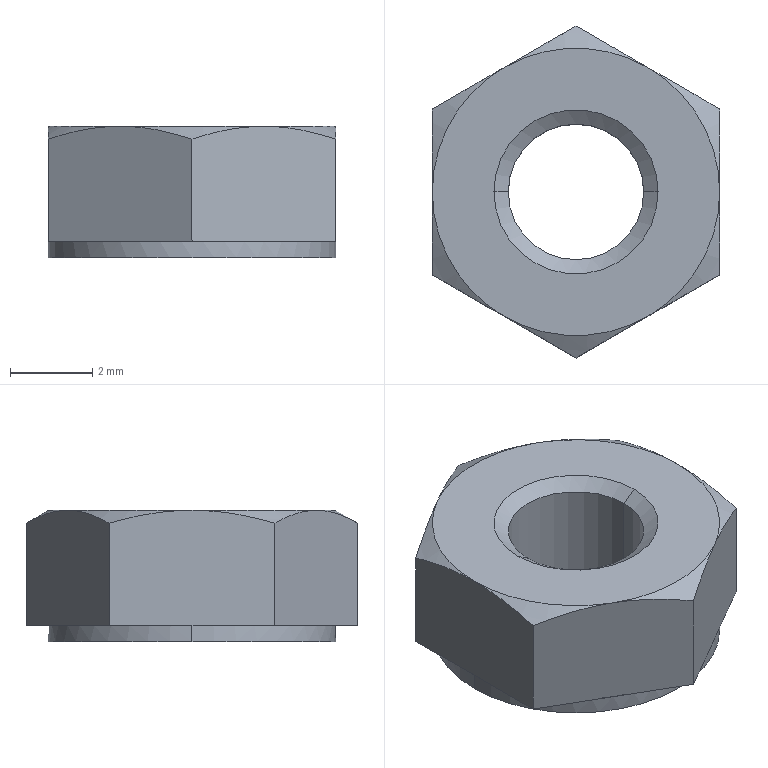Part | SolidWorks | features RevCut 4, Extrusion 1, LPattern 1 | 1 solid | 30 faces | box 7 x 8.083 x 3.2 mm | volume 105.415 mm3 | plane 14 | cone 10 | cylinder 6 | commonest cylinder face diameters 3.3 x2 4 x2 7 x2
STEP:
#1=CARTESIAN_POINT('',(-2.,0.,-3.2));
#2=VERTEX_POINT('',#1);
#3=CARTESIAN_POINT('',(2.,0.,-3.2));
#4=VERTEX_POINT('',#3);
#5=CARTESIAN_POINT('',(0.,0.,-3.2));
#6=DIRECTION('',(0.,0.,1.));
#7=DIRECTION('',(-1.,0.,0.));
#8=AXIS2_PLACEMENT_3D('',#5,#6,#7);
#9=CIRCLE('',#8,2.);
#10=EDGE_CURVE('',#2,#4,#9,.T.);
#11=ORIENTED_EDGE('',*,*,#10,.F.);
#12=CARTESIAN_POINT('',(-2.,0.,-3.175));
#13=VERTEX_POINT('',#12);
#14=CARTESIAN_POINT('',(-2.,0.,-25.038));
#15=DIRECTION('',(0.,0.,1.));
#16=VECTOR('',#15,1000.);
#17=LINE('',#14,#16);
#18=EDGE_CURVE('',#2,#13,#17,.T.);
#19=ORIENTED_EDGE('',*,*,#18,.T.);
#20=CARTESIAN_POINT('',(2.,0.,-3.175));
#21=VERTEX_POINT('',#20);
#22=CARTESIAN_POINT('',(0.,0.,-3.175));
#23=DIRECTION('',(0.,0.,1.));
#24=DIRECTION('',(1.,0.,0.));
#25=AXIS2_PLACEMENT_3D('',#22,#23,#24);
#26=CIRCLE('',#25,2.);
#27=EDGE_CURVE('',#13,#21,#26,.T.);
#28=ORIENTED_EDGE('',*,*,#27,.T.);
#29=CARTESIAN_POINT('',(2.,0.,-25.038));
#30=DIRECTION('',(0.,0.,1.));
#31=VECTOR('',#30,1000.);
#32=LINE('',#29,#31);
#33=EDGE_CURVE('',#4,#21,#32,.T.);
#34=ORIENTED_EDGE('',*,*,#33,.F.);
#35=EDGE_LOOP('',(#11,#19,#28,#34));
#36=FACE_OUTER_BOUND('',#35,.T.);
#37=CARTESIAN_POINT('',(0.,0.,-25.038));
#38=DIRECTION('',(0.,0.,1.));
#39=DIRECTION('',(1.,0.,0.));
#40=AXIS2_PLACEMENT_3D('',#37,#38,#39);
#41=CYLINDRICAL_SURFACE('',#40,2.);
#42=ADVANCED_FACE('',(#36),#41,.F.);
#43=CARTESIAN_POINT('',(-1.65,0.,-2.93));
#44=VERTEX_POINT('',#43);
#45=CARTESIAN_POINT('',(1.65,0.,-2.93));
#46=VERTEX_POINT('',#45);
#47=CARTESIAN_POINT('',(0.,0.,-2.93));
#48=DIRECTION('',(0.,0.,1.));
#49=DIRECTION('',(-1.,0.,0.));
#50=AXIS2_PLACEMENT_3D('',#47,#48,#49);
#51=CIRCLE('',#50,1.65);
#52=EDGE_CURVE('',#44,#46,#51,.T.);
#53=ORIENTED_EDGE('',*,*,#52,.T.);
#54=CARTESIAN_POINT('',(2.,0.,-3.175));
#55=DIRECTION('',(0.8192,0.,-0.5736));
#56=VECTOR('',#55,1000.);
#57=LINE('',#54,#56);
#58=EDGE_CURVE('',#46,#21,#57,.T.);
#59=ORIENTED_EDGE('',*,*,#58,.T.);
#60=ORIENTED_EDGE('',*,*,#27,.F.);
#61=CARTESIAN_POINT('',(-2.,0.,-3.175));
#62=DIRECTION('',(-0.8192,0.,-0.5736));
#63=VECTOR('',#62,1000.);
#64=LINE('',#61,#63);
#65=EDGE_CURVE('',#44,#13,#64,.T.);
#66=ORIENTED_EDGE('',*,*,#65,.F.);
#67=EDGE_LOOP('',(#53,#59,#60,#66));
#68=FACE_OUTER_BOUND('',#67,.T.);
#69=CARTESIAN_POINT('',(0.,0.,-3.175));
#70=DIRECTION('',(0.,0.,-1.));
#71=DIRECTION('',(-1.,0.,0.));
#72=AXIS2_PLACEMENT_3D('',#69,#70,#71);
#73=CONICAL_SURFACE('',#72,2.,0.9599);
#74=ADVANCED_FACE('',(#68),#73,.F.);
#75=CARTESIAN_POINT('',(1.65,0.,-0.2451));
#76=VERTEX_POINT('',#75);
#77=CARTESIAN_POINT('',(-1.65,0.,-0.2451));
#78=VERTEX_POINT('',#77);
#79=CARTESIAN_POINT('',(0.,0.,-0.2451));
#80=DIRECTION('',(0.,0.,-1.));
#81=DIRECTION('',(1.,0.,0.));
#82=AXIS2_PLACEMENT_3D('',#79,#80,#81);
#83=CIRCLE('',#82,1.65);
#84=EDGE_CURVE('',#76,#78,#83,.T.);
#85=ORIENTED_EDGE('',*,*,#84,.T.);
#86=CARTESIAN_POINT('',(-2.,0.,0.));
#87=VERTEX_POINT('',#86);
#88=CARTESIAN_POINT('',(-1.615,0.,-0.2696));
#89=DIRECTION('',(-0.8192,0.,0.5736));
#90=VECTOR('',#89,1000.);
#91=LINE('',#88,#90);
#92=EDGE_CURVE('',#78,#87,#91,.T.);
#93=ORIENTED_EDGE('',*,*,#92,.T.);
#94=CARTESIAN_POINT('',(2.,0.,0.));
#95=VERTEX_POINT('',#94);
#96=CARTESIAN_POINT('',(0.,0.,0.));
#97=DIRECTION('',(0.,0.,1.));
#98=DIRECTION('',(1.,0.,0.));
#99=AXIS2_PLACEMENT_3D('',#96,#97,#98);
#100=CIRCLE('',#99,2.);
#101=EDGE_CURVE('',#87,#95,#100,.T.);
#102=ORIENTED_EDGE('',*,*,#101,.T.);
#103=CARTESIAN_POINT('',(1.615,0.,-0.2696));
#104=DIRECTION('',(0.8192,0.,0.5736));
#105=VECTOR('',#104,1000.);
#106=LINE('',#103,#105);
#107=EDGE_CURVE('',#76,#95,#106,.T.);
#108=ORIENTED_EDGE('',*,*,#107,.F.);
#109=EDGE_LOOP('',(#85,#93,#102,#108));
#110=FACE_OUTER_BOUND('',#109,.T.);
#111=CARTESIAN_POINT('',(0.,0.,-0.2696));
#112=DIRECTION('',(0.,0.,1.));
#113=DIRECTION('',(1.,0.,0.));
#114=AXIS2_PLACEMENT_3D('',#111,#112,#113);
#115=CONICAL_SURFACE('',#114,1.615,0.9599);
#116=ADVANCED_FACE('',(#110),#115,.F.);
#117=CARTESIAN_POINT('',(3.5,0.,-3.2));
#118=VERTEX_POINT('',#117);
#119=CARTESIAN_POINT('',(-3.5,0.,-3.2));
#120=VERTEX_POINT('',#119);
#121=CARTESIAN_POINT('',(0.,0.,-3.2));
#122=DIRECTION('',(0.,0.,1.));
#123=DIRECTION('',(-1.,0.,0.));
#124=AXIS2_PLACEMENT_3D('',#121,#122,#123);
#125=CIRCLE('',#124,3.5);
#126=EDGE_CURVE('',#118,#120,#125,.T.);
#127=ORIENTED_EDGE('',*,*,#126,.T.);
#128=CARTESIAN_POINT('',(-3.5,0.,-2.8));
#129=VERTEX_POINT('',#128);
#130=CARTESIAN_POINT('',(-3.5,0.,0.));
#131=DIRECTION('',(0.,0.,1.));
#132=VECTOR('',#131,1000.);
#133=LINE('',#130,#132);
#134=EDGE_CURVE('',#120,#129,#133,.T.);
#135=ORIENTED_EDGE('',*,*,#134,.T.);
#136=CARTESIAN_POINT('',(-1.75,3.031,-2.8));
#137=VERTEX_POINT('',#136);
#138=CARTESIAN_POINT('',(0.,0.,-2.8));
#139=DIRECTION('',(0.,0.,1.));
#140=DIRECTION('',(1.,0.,0.));
#141=AXIS2_PLACEMENT_3D('',#138,#139,#140);
#142=CIRCLE('',#141,3.5);
#143=EDGE_CURVE('',#137,#129,#142,.T.);
#144=ORIENTED_EDGE('',*,*,#143,.F.);
#145=CARTESIAN_POINT('',(1.75,3.031,-2.8));
#146=VERTEX_POINT('',#145);
#147=CARTESIAN_POINT('',(0.,0.,-2.8));
#148=DIRECTION('',(0.,0.,1.));
#149=DIRECTION('',(1.,0.,0.));
#150=AXIS2_PLACEMENT_3D('',#147,#148,#149);
#151=CIRCLE('',#150,3.5);
#152=EDGE_CURVE('',#146,#137,#151,.T.);
#153=ORIENTED_EDGE('',*,*,#152,.F.);
#154=CARTESIAN_POINT('',(3.5,0.,-2.8));
#155=VERTEX_POINT('',#154);
#156=CARTESIAN_POINT('',(0.,0.,-2.8));
#157=DIRECTION('',(0.,0.,1.));
#158=DIRECTION('',(1.,0.,0.));
#159=AXIS2_PLACEMENT_3D('',#156,#157,#158);
#160=CIRCLE('',#159,3.5);
#161=EDGE_CURVE('',#155,#146,#160,.T.);
#162=ORIENTED_EDGE('',*,*,#161,.F.);
#163=CARTESIAN_POINT('',(3.5,0.,0.));
#164=DIRECTION('',(0.,0.,1.));
#165=VECTOR('',#164,1000.);
#166=LINE('',#163,#165);
#167=EDGE_CURVE('',#118,#155,#166,.T.);
#168=ORIENTED_EDGE('',*,*,#167,.F.);
#169=EDGE_LOOP('',(#127,#135,#144,#153,#162,#168));
#170=FACE_OUTER_BOUND('',#169,.T.);
#171=CARTESIAN_POINT('',(0.,0.,0.));
#172=DIRECTION('',(0.,0.,1.));
#173=DIRECTION('',(1.,0.,0.));
#174=AXIS2_PLACEMENT_3D('',#171,#172,#173);
#175=CYLINDRICAL_SURFACE('',#174,3.5);
#176=ADVANCED_FACE('',(#170),#175,.T.);
#177=ORIENTED_EDGE('',*,*,#52,.F.);
#178=CARTESIAN_POINT('',(-1.65,0.,-3.2));
#179=DIRECTION('',(0.,0.,1.));
#180=VECTOR('',#179,1000.);
#181=LINE('',#178,#180);
#182=EDGE_CURVE('',#44,#78,#181,.T.);
#183=ORIENTED_EDGE('',*,*,#182,.T.);
#184=ORIENTED_EDGE('',*,*,#84,.F.);
#185=CARTESIAN_POINT('',(1.65,0.,-3.2));
#186=DIRECTION('',(0.,0.,1.));
#187=VECTOR('',#186,1000.);
#188=LINE('',#185,#187);
#189=EDGE_CURVE('',#46,#76,#188,.T.);
#190=ORIENTED_EDGE('',*,*,#189,.F.);
#191=EDGE_LOOP('',(#177,#183,#184,#190));
#192=FACE_OUTER_BOUND('',#191,.T.);
#193=CARTESIAN_POINT('',(0.,0.,-3.2));
#194=DIRECTION('',(0.,0.,1.));
#195=DIRECTION('',(1.,0.,0.));
#196=AXIS2_PLACEMENT_3D('',#193,#194,#195);
#197=CYLINDRICAL_SURFACE('',#196,1.65);
#198=ADVANCED_FACE('',(#192),#197,.F.);
#199=ORIENTED_EDGE('',*,*,#182,.F.);
#200=CARTESIAN_POINT('',(0.,0.,-2.93));
#201=DIRECTION('',(0.,0.,1.));
#202=DIRECTION('',(-1.,0.,0.));
#203=AXIS2_PLACEMENT_3D('',#200,#201,#202);
#204=CIRCLE('',#203,1.65);
#205=EDGE_CURVE('',#46,#44,#204,.T.);
#206=ORIENTED_EDGE('',*,*,#205,.F.);
#207=ORIENTED_EDGE('',*,*,#189,.T.);
#208=CARTESIAN_POINT('',(0.,0.,-0.2451));
#209=DIRECTION('',(0.,0.,-1.));
#210=DIRECTION('',(1.,0.,0.));
#211=AXIS2_PLACEMENT_3D('',#208,#209,#210);
#212=CIRCLE('',#211,1.65);
#213=EDGE_CURVE('',#78,#76,#212,.T.);
#214=ORIENTED_EDGE('',*,*,#213,.F.);
#215=EDGE_LOOP('',(#199,#206,#207,#214));
#216=FACE_OUTER_BOUND('',#215,.T.);
#217=CARTESIAN_POINT('',(0.,0.,-3.2));
#218=DIRECTION('',(0.,0.,1.));
#219=DIRECTION('',(1.,0.,0.));
#220=AXIS2_PLACEMENT_3D('',#217,#218,#219);
#221=CYLINDRICAL_SURFACE('',#220,1.65);
#222=ADVANCED_FACE('',(#216),#221,.F.);
#223=CARTESIAN_POINT('',(-3.5,2.021,-2.8));
#224=VERTEX_POINT('',#223);
#225=CARTESIAN_POINT('',(-3.5,2.021,-0.3126));
#226=VERTEX_POINT('',#225);
#227=CARTESIAN_POINT('',(-3.5,2.021,-3.2));
#228=DIRECTION('',(0.,0.,1.));
#229=VECTOR('',#228,1000.);
#230=LINE('',#227,#229);
#231=EDGE_CURVE('',#224,#226,#230,.T.);
#232=ORIENTED_EDGE('',*,*,#231,.T.);
#233=CARTESIAN_POINT('',(-1.75,3.031,0.));
#234=VERTEX_POINT('',#233);
#235=CARTESIAN_POINT('',(-3.5,2.021,-0.3126));
#236=CARTESIAN_POINT('',(-2.927,2.351,-0.1218));
#237=CARTESIAN_POINT('',(-2.346,2.687,0.));
#238=CARTESIAN_POINT('',(-1.75,3.031,0.));
#239=B_SPLINE_CURVE_WITH_KNOTS('',3,(#235,#236,#237,#238),.UNSPECIFIED.,.F.,.F.,(4,4),(0.000000238,0.002045),.UNSPECIFIED.);
#240=EDGE_CURVE('',#226,#234,#239,.T.);
#241=ORIENTED_EDGE('',*,*,#240,.T.);
#242=CARTESIAN_POINT('',(0.,4.041,-0.3126));
#243=VERTEX_POINT('',#242);
#244=CARTESIAN_POINT('',(-1.75,3.031,0.));
#245=CARTESIAN_POINT('',(-1.453,3.203,0.));
#246=CARTESIAN_POINT('',(-1.156,3.374,-0.02993));
#247=CARTESIAN_POINT('',(-0.5735,3.71,-0.1388));
#248=CARTESIAN_POINT('',(-0.2856,3.877,-0.2174));
#249=CARTESIAN_POINT('',(0.,4.041,-0.3126));
#250=B_SPLINE_CURVE_WITH_KNOTS('',3,(#244,#245,#246,#247,#248,#249),.UNSPECIFIED.,.F.,.F.,(4,2,4),(0.002045,0.003063,0.004082),.UNSPECIFIED.);
#251=EDGE_CURVE('',#234,#243,#250,.T.);
#252=ORIENTED_EDGE('',*,*,#251,.T.);
#253=CARTESIAN_POINT('',(0.,4.041,-2.8));
#254=VERTEX_POINT('',#253);
#255=CARTESIAN_POINT('',(0.,4.041,-3.2));
#256=DIRECTION('',(0.,0.,1.));
#257=VECTOR('',#256,1000.);
#258=LINE('',#255,#257);
#259=EDGE_CURVE('',#254,#243,#258,.T.);
#260=ORIENTED_EDGE('',*,*,#259,.F.);
#261=CARTESIAN_POINT('',(0.,4.041,-2.8));
#262=DIRECTION('',(-0.866,-0.5,0.));
#263=VECTOR('',#262,1000.);
#264=LINE('',#261,#263);
#265=EDGE_CURVE('',#254,#137,#264,.T.);
#266=ORIENTED_EDGE('',*,*,#265,.T.);
#267=CARTESIAN_POINT('',(0.,4.041,-2.8));
#268=DIRECTION('',(-0.866,-0.5,0.));
#269=VECTOR('',#268,1000.);
#270=LINE('',#267,#269);
#271=EDGE_CURVE('',#137,#224,#270,.T.);
#272=ORIENTED_EDGE('',*,*,#271,.T.);
#273=EDGE_LOOP('',(#232,#241,#252,#260,#266,#272));
#274=FACE_OUTER_BOUND('',#273,.T.);
#275=CARTESIAN_POINT('',(0.,4.041,-3.2));
#276=DIRECTION('',(-0.5,0.866,0.));
#277=DIRECTION('',(-0.866,-0.5,0.));
#278=AXIS2_PLACEMENT_3D('',#275,#276,#277);
#279=PLANE('',#278);
#280=ADVANCED_FACE('',(#274),#279,.T.);
#281=ORIENTED_EDGE('',*,*,#259,.T.);
#282=CARTESIAN_POINT('',(1.75,3.031,0.));
#283=VERTEX_POINT('',#282);
#284=CARTESIAN_POINT('',(0.,4.041,-0.3126));
#285=CARTESIAN_POINT('',(0.5726,3.711,-0.1218));
#286=CARTESIAN_POINT('',(1.154,3.375,0.));
#287=CARTESIAN_POINT('',(1.75,3.031,0.));
#288=B_SPLINE_CURVE_WITH_KNOTS('',3,(#284,#285,#286,#287),.UNSPECIFIED.,.F.,.F.,(4,4),(0.000000238,0.002045),.UNSPECIFIED.);
#289=EDGE_CURVE('',#243,#283,#288,.T.);
#290=ORIENTED_EDGE('',*,*,#289,.T.);
#291=CARTESIAN_POINT('',(3.5,2.021,-0.3126));
#292=VERTEX_POINT('',#291);
#293=CARTESIAN_POINT('',(1.75,3.031,0.));
#294=CARTESIAN_POINT('',(2.047,2.86,0.));
#295=CARTESIAN_POINT('',(2.344,2.688,-0.02993));
#296=CARTESIAN_POINT('',(2.926,2.352,-0.1388));
#297=CARTESIAN_POINT('',(3.214,2.186,-0.2174));
#298=CARTESIAN_POINT('',(3.5,2.021,-0.3126));
#299=B_SPLINE_CURVE_WITH_KNOTS('',3,(#293,#294,#295,#296,#297,#298),.UNSPECIFIED.,.F.,.F.,(4,2,4),(0.002045,0.003063,0.004082),.UNSPECIFIED.);
#300=EDGE_CURVE('',#283,#292,#299,.T.);
#301=ORIENTED_EDGE('',*,*,#300,.T.);
#302=CARTESIAN_POINT('',(3.5,2.021,-2.8));
#303=VERTEX_POINT('',#302);
#304=CARTESIAN_POINT('',(3.5,2.021,-3.2));
#305=DIRECTION('',(0.,0.,1.));
#306=VECTOR('',#305,1000.);
#307=LINE('',#304,#306);
#308=EDGE_CURVE('',#303,#292,#307,.T.);
#309=ORIENTED_EDGE('',*,*,#308,.F.);
#310=CARTESIAN_POINT('',(3.5,2.021,-2.8));
#311=DIRECTION('',(-0.866,0.5,0.));
#312=VECTOR('',#311,1000.);
#313=LINE('',#310,#312);
#314=EDGE_CURVE('',#303,#146,#313,.T.);
#315=ORIENTED_EDGE('',*,*,#314,.T.);
#316=CARTESIAN_POINT('',(3.5,2.021,-2.8));
#317=DIRECTION('',(-0.866,0.5,0.));
#318=VECTOR('',#317,1000.);
#319=LINE('',#316,#318);
#320=EDGE_CURVE('',#146,#254,#319,.T.);
#321=ORIENTED_EDGE('',*,*,#320,.T.);
#322=EDGE_LOOP('',(#281,#290,#301,#309,#315,#321));
#323=FACE_OUTER_BOUND('',#322,.T.);
#324=CARTESIAN_POINT('',(3.5,2.021,-3.2));
#325=DIRECTION('',(0.5,0.866,0.));
#326=DIRECTION('',(-0.866,0.5,0.));
#327=AXIS2_PLACEMENT_3D('',#324,#325,#326);
#328=PLANE('',#327);
#329=ADVANCED_FACE('',(#323),#328,.T.);
#330=CARTESIAN_POINT('',(3.5,-2.021,-0.3126));
#331=VERTEX_POINT('',#330);
#332=CARTESIAN_POINT('',(3.5,0.,0.));
#333=VERTEX_POINT('',#332);
#334=CARTESIAN_POINT('',(3.5,-2.021,-0.3126));
#335=CARTESIAN_POINT('',(3.5,-1.692,-0.2177));
#336=CARTESIAN_POINT('',(3.5,-1.355,-0.1382));
#337=CARTESIAN_POINT('',(3.5,-0.6807,-0.02935));
#338=CARTESIAN_POINT('',(3.5,-0.3415,0.));
#339=CARTESIAN_POINT('',(3.5,0.,0.));
#340=B_SPLINE_CURVE_WITH_KNOTS('',3,(#334,#335,#336,#337,#338,#339),.UNSPECIFIED.,.F.,.F.,(4,2,4),(0.003605,0.004627,0.005649),.UNSPECIFIED.);
#341=EDGE_CURVE('',#331,#333,#340,.T.);
#342=ORIENTED_EDGE('',*,*,#341,.F.);
#343=CARTESIAN_POINT('',(3.5,-2.021,-2.8));
#344=VERTEX_POINT('',#343);
#345=CARTESIAN_POINT('',(3.5,-2.021,-3.2));
#346=DIRECTION('',(0.,0.,1.));
#347=VECTOR('',#346,1000.);
#348=LINE('',#345,#347);
#349=EDGE_CURVE('',#344,#331,#348,.T.);
#350=ORIENTED_EDGE('',*,*,#349,.F.);
#351=CARTESIAN_POINT('',(3.5,2.021,-2.8));
#352=DIRECTION('',(0.,-1.,0.));
#353=VECTOR('',#352,1000.);
#354=LINE('',#351,#353);
#355=EDGE_CURVE('',#155,#344,#354,.T.);
#356=ORIENTED_EDGE('',*,*,#355,.F.);
#357=CARTESIAN_POINT('',(3.5,2.021,-2.8));
#358=DIRECTION('',(0.,-1.,0.));
#359=VECTOR('',#358,1000.);
#360=LINE('',#357,#359);
#361=EDGE_CURVE('',#303,#155,#360,.T.);
#362=ORIENTED_EDGE('',*,*,#361,.F.);
#363=ORIENTED_EDGE('',*,*,#308,.T.);
#364=CARTESIAN_POINT('',(3.5,0.,0.));
#365=CARTESIAN_POINT('',(3.5,0.3417,0.));
#366=CARTESIAN_POINT('',(3.5,0.688,-0.03016));
#367=CARTESIAN_POINT('',(3.5,1.363,-0.1397));
#368=CARTESIAN_POINT('',(3.5,1.694,-0.2183));
#369=CARTESIAN_POINT('',(3.5,2.021,-0.3126));
#370=B_SPLINE_CURVE_WITH_KNOTS('',3,(#364,#365,#366,#367,#368,#369),.UNSPECIFIED.,.F.,.F.,(4,2,4),(0.005649,0.006672,0.007695),.UNSPECIFIED.);
#371=EDGE_CURVE('',#333,#292,#370,.T.);
#372=ORIENTED_EDGE('',*,*,#371,.F.);
#373=EDGE_LOOP('',(#342,#350,#356,#362,#363,#372));
#374=FACE_OUTER_BOUND('',#373,.T.);
#375=CARTESIAN_POINT('',(3.5,2.021,-3.2));
#376=DIRECTION('',(-1.,0.,0.));
#377=DIRECTION('',(0.,0.,1.));
#378=AXIS2_PLACEMENT_3D('',#375,#376,#377);
#379=PLANE('',#378);
#380=ADVANCED_FACE('',(#374),#379,.F.);
#381=ORIENTED_EDGE('',*,*,#349,.T.);
#382=CARTESIAN_POINT('',(1.75,-3.031,0.));
#383=VERTEX_POINT('',#382);
#384=CARTESIAN_POINT('',(3.5,-2.021,-0.3126));
#385=CARTESIAN_POINT('',(2.927,-2.351,-0.1218));
#386=CARTESIAN_POINT('',(2.346,-2.687,0.));
#387=CARTESIAN_POINT('',(1.75,-3.031,0.));
#388=B_SPLINE_CURVE_WITH_KNOTS('',3,(#384,#385,#386,#387),.UNSPECIFIED.,.F.,.F.,(4,4),(0.000000238,0.002045),.UNSPECIFIED.);
#389=EDGE_CURVE('',#331,#383,#388,.T.);
#390=ORIENTED_EDGE('',*,*,#389,.T.);
#391=CARTESIAN_POINT('',(0.,-4.041,-0.3126));
#392=VERTEX_POINT('',#391);
#393=CARTESIAN_POINT('',(1.75,-3.031,0.));
#394=CARTESIAN_POINT('',(1.453,-3.203,0.));
#395=CARTESIAN_POINT('',(1.156,-3.374,-0.02993));
#396=CARTESIAN_POINT('',(0.5735,-3.71,-0.1388));
#397=CARTESIAN_POINT('',(0.2856,-3.877,-0.2174));
#398=CARTESIAN_POINT('',(0.,-4.041,-0.3126));
#399=B_SPLINE_CURVE_WITH_KNOTS('',3,(#393,#394,#395,#396,#397,#398),.UNSPECIFIED.,.F.,.F.,(4,2,4),(0.002045,0.003063,0.004082),.UNSPECIFIED.);
#400=EDGE_CURVE('',#383,#392,#399,.T.);
#401=ORIENTED_EDGE('',*,*,#400,.T.);
#402=CARTESIAN_POINT('',(0.,-4.041,-2.8));
#403=VERTEX_POINT('',#402);
#404=CARTESIAN_POINT('',(0.,-4.041,-3.2));
#405=DIRECTION('',(0.,0.,1.));
#406=VECTOR('',#405,1000.);
#407=LINE('',#404,#406);
#408=EDGE_CURVE('',#403,#392,#407,.T.);
#409=ORIENTED_EDGE('',*,*,#408,.F.);
#410=CARTESIAN_POINT('',(1.75,-3.031,-2.8));
#411=VERTEX_POINT('',#410);
#412=CARTESIAN_POINT('',(0.,-4.041,-2.8));
#413=DIRECTION('',(0.866,0.5,0.));
#414=VECTOR('',#413,1000.);
#415=LINE('',#412,#414);
#416=EDGE_CURVE('',#403,#411,#415,.T.);
#417=ORIENTED_EDGE('',*,*,#416,.T.);
#418=CARTESIAN_POINT('',(0.,-4.041,-2.8));
#419=DIRECTION('',(0.866,0.5,0.));
#420=VECTOR('',#419,1000.);
#421=LINE('',#418,#420);
#422=EDGE_CURVE('',#411,#344,#421,.T.);
#423=ORIENTED_EDGE('',*,*,#422,.T.);
#424=EDGE_LOOP('',(#381,#390,#401,#409,#417,#423));
#425=FACE_OUTER_BOUND('',#424,.T.);
#426=CARTESIAN_POINT('',(0.,-4.041,-3.2));
#427=DIRECTION('',(0.5,-0.866,0.));
#428=DIRECTION('',(0.866,0.5,0.));
#429=AXIS2_PLACEMENT_3D('',#426,#427,#428);
#430=PLANE('',#429);
#431=ADVANCED_FACE('',(#425),#430,.T.);
#432=ORIENTED_EDGE('',*,*,#408,.T.);
#433=CARTESIAN_POINT('',(-1.75,-3.031,0.));
#434=VERTEX_POINT('',#433);
#435=CARTESIAN_POINT('',(0.,-4.041,-0.3126));
#436=CARTESIAN_POINT('',(-0.5726,-3.711,-0.1218));
#437=CARTESIAN_POINT('',(-1.154,-3.375,0.));
#438=CARTESIAN_POINT('',(-1.75,-3.031,0.));
#439=B_SPLINE_CURVE_WITH_KNOTS('',3,(#435,#436,#437,#438),.UNSPECIFIED.,.F.,.F.,(4,4),(0.000000238,0.002045),.UNSPECIFIED.);
#440=EDGE_CURVE('',#392,#434,#439,.T.);
#441=ORIENTED_EDGE('',*,*,#440,.T.);
#442=CARTESIAN_POINT('',(-3.5,-2.021,-0.3126));
#443=VERTEX_POINT('',#442);
#444=CARTESIAN_POINT('',(-1.75,-3.031,0.));
#445=CARTESIAN_POINT('',(-2.047,-2.86,0.));
#446=CARTESIAN_POINT('',(-2.344,-2.688,-0.02993));
#447=CARTESIAN_POINT('',(-2.926,-2.352,-0.1388));
#448=CARTESIAN_POINT('',(-3.214,-2.186,-0.2174));
#449=CARTESIAN_POINT('',(-3.5,-2.021,-0.3126));
#450=B_SPLINE_CURVE_WITH_KNOTS('',3,(#444,#445,#446,#447,#448,#449),.UNSPECIFIED.,.F.,.F.,(4,2,4),(0.002045,0.003063,0.004082),.UNSPECIFIED.);
#451=EDGE_CURVE('',#434,#443,#450,.T.);
#452=ORIENTED_EDGE('',*,*,#451,.T.);
#453=CARTESIAN_POINT('',(-3.5,-2.021,-2.8));
#454=VERTEX_POINT('',#453);
#455=CARTESIAN_POINT('',(-3.5,-2.021,-3.2));
#456=DIRECTION('',(0.,0.,1.));
#457=VECTOR('',#456,1000.);
#458=LINE('',#455,#457);
#459=EDGE_CURVE('',#454,#443,#458,.T.);
#460=ORIENTED_EDGE('',*,*,#459,.F.);
#461=CARTESIAN_POINT('',(-1.75,-3.031,-2.8));
#462=VERTEX_POINT('',#461);
#463=CARTESIAN_POINT('',(-3.5,-2.021,-2.8));
#464=DIRECTION('',(0.866,-0.5,0.));
#465=VECTOR('',#464,1000.);
#466=LINE('',#463,#465);
#467=EDGE_CURVE('',#454,#462,#466,.T.);
#468=ORIENTED_EDGE('',*,*,#467,.T.);
#469=CARTESIAN_POINT('',(-3.5,-2.021,-2.8));
#470=DIRECTION('',(0.866,-0.5,0.));
#471=VECTOR('',#470,1000.);
#472=LINE('',#469,#471);
#473=EDGE_CURVE('',#462,#403,#472,.T.);
#474=ORIENTED_EDGE('',*,*,#473,.T.);
#475=EDGE_LOOP('',(#432,#441,#452,#460,#468,#474));
#476=FACE_OUTER_BOUND('',#475,.T.);
#477=CARTESIAN_POINT('',(-3.5,-2.021,-3.2));
#478=DIRECTION('',(-0.5,-0.866,0.));
#479=DIRECTION('',(0.866,-0.5,0.));
#480=AXIS2_PLACEMENT_3D('',#477,#478,#479);
#481=PLANE('',#480);
#482=ADVANCED_FACE('',(#476),#481,.T.);
#483=ORIENTED_EDGE('',*,*,#459,.T.);
#484=CARTESIAN_POINT('',(-3.5,0.,0.));
#485=VERTEX_POINT('',#484);
#486=CARTESIAN_POINT('',(-3.5,-2.021,-0.3126));
#487=CARTESIAN_POINT('',(-3.5,-1.692,-0.2177));
#488=CARTESIAN_POINT('',(-3.5,-1.355,-0.1382));
#489=CARTESIAN_POINT('',(-3.5,-0.6807,-0.02935));
#490=CARTESIAN_POINT('',(-3.5,-0.3415,0.));
#491=CARTESIAN_POINT('',(-3.5,0.,0.));
#492=B_SPLINE_CURVE_WITH_KNOTS('',3,(#486,#487,#488,#489,#490,#491),.UNSPECIFIED.,.F.,.F.,(4,2,4),(0.003605,0.004627,0.005649),.UNSPECIFIED.);
#493=EDGE_CURVE('',#443,#485,#492,.T.);
#494=ORIENTED_EDGE('',*,*,#493,.T.);
#495=CARTESIAN_POINT('',(-3.5,0.,0.));
#496=CARTESIAN_POINT('',(-3.5,0.3417,0.));
#497=CARTESIAN_POINT('',(-3.5,0.688,-0.03016));
#498=CARTESIAN_POINT('',(-3.5,1.363,-0.1397));
#499=CARTESIAN_POINT('',(-3.5,1.694,-0.2183));
#500=CARTESIAN_POINT('',(-3.5,2.021,-0.3126));
#501=B_SPLINE_CURVE_WITH_KNOTS('',3,(#495,#496,#497,#498,#499,#500),.UNSPECIFIED.,.F.,.F.,(4,2,4),(0.005649,0.006672,0.007695),.UNSPECIFIED.);
#502=EDGE_CURVE('',#485,#226,#501,.T.);
#503=ORIENTED_EDGE('',*,*,#502,.T.);
#504=ORIENTED_EDGE('',*,*,#231,.F.);
#505=CARTESIAN_POINT('',(-3.5,2.021,-2.8));
#506=DIRECTION('',(0.,-1.,0.));
#507=VECTOR('',#506,1000.);
#508=LINE('',#505,#507);
#509=EDGE_CURVE('',#224,#129,#508,.T.);
#510=ORIENTED_EDGE('',*,*,#509,.T.);
#511=CARTESIAN_POINT('',(-3.5,2.021,-2.8));
#512=DIRECTION('',(0.,-1.,0.));
#513=VECTOR('',#512,1000.);
#514=LINE('',#511,#513);
#515=EDGE_CURVE('',#129,#454,#514,.T.);
#516=ORIENTED_EDGE('',*,*,#515,.T.);
#517=EDGE_LOOP('',(#483,#494,#503,#504,#510,#516));
#518=FACE_OUTER_BOUND('',#517,.T.);
#519=CARTESIAN_POINT('',(-3.5,2.021,-3.2));
#520=DIRECTION('',(-1.,0.,0.));
#521=DIRECTION('',(0.,0.,1.));
#522=AXIS2_PLACEMENT_3D('',#519,#520,#521);
#523=PLANE('',#522);
#524=ADVANCED_FACE('',(#518),#523,.T.);
#525=CARTESIAN_POINT('',(0.,0.,0.));
#526=DIRECTION('',(0.,0.,1.));
#527=DIRECTION('',(1.,0.,0.));
#528=AXIS2_PLACEMENT_3D('',#525,#526,#527);
#529=CIRCLE('',#528,2.);
#530=EDGE_CURVE('',#95,#87,#529,.T.);
#531=ORIENTED_EDGE('',*,*,#530,.F.);
#532=ORIENTED_EDGE('',*,*,#101,.F.);
#533=EDGE_LOOP('',(#531,#532));
#534=FACE_BOUND('',#533,.T.);
#535=CARTESIAN_POINT('',(0.,0.,0.));
#536=DIRECTION('',(0.,0.,1.));
#537=DIRECTION('',(-1.,0.,0.));
#538=AXIS2_PLACEMENT_3D('',#535,#536,#537);
#539=CIRCLE('',#538,3.5);
#540=EDGE_CURVE('',#234,#485,#539,.T.);
#541=ORIENTED_EDGE('',*,*,#540,.T.);
#542=CARTESIAN_POINT('',(0.,0.,0.));
#543=DIRECTION('',(0.,0.,1.));
#544=DIRECTION('',(-1.,0.,0.));
#545=AXIS2_PLACEMENT_3D('',#542,#543,#544);
#546=CIRCLE('',#545,3.5);
#547=EDGE_CURVE('',#485,#434,#546,.T.);
#548=ORIENTED_EDGE('',*,*,#547,.T.);
#549=CARTESIAN_POINT('',(0.,0.,0.));
#550=DIRECTION('',(0.,0.,1.));
#551=DIRECTION('',(-1.,0.,0.));
#552=AXIS2_PLACEMENT_3D('',#549,#550,#551);
#553=CIRCLE('',#552,3.5);
#554=EDGE_CURVE('',#434,#383,#553,.T.);
#555=ORIENTED_EDGE('',*,*,#554,.T.);
#556=CARTESIAN_POINT('',(0.,0.,0.));
#557=DIRECTION('',(0.,0.,1.));
#558=DIRECTION('',(-1.,0.,0.));
#559=AXIS2_PLACEMENT_3D('',#556,#557,#558);
#560=CIRCLE('',#559,3.5);
#561=EDGE_CURVE('',#383,#333,#560,.T.);
#562=ORIENTED_EDGE('',*,*,#561,.T.);
#563=CARTESIAN_POINT('',(0.,0.,0.));
#564=DIRECTION('',(0.,0.,1.));
#565=DIRECTION('',(1.,0.,0.));
#566=AXIS2_PLACEMENT_3D('',#563,#564,#565);
#567=CIRCLE('',#566,3.5);
#568=EDGE_CURVE('',#333,#283,#567,.T.);
#569=ORIENTED_EDGE('',*,*,#568,.T.);
#570=CARTESIAN_POINT('',(0.,0.,0.));
#571=DIRECTION('',(0.,0.,1.));
#572=DIRECTION('',(-1.,0.,0.));
#573=AXIS2_PLACEMENT_3D('',#570,#571,#572);
#574=CIRCLE('',#573,3.5);
#575=EDGE_CURVE('',#283,#234,#574,.T.);
#576=ORIENTED_EDGE('',*,*,#575,.T.);
#577=EDGE_LOOP('',(#541,#548,#555,#562,#569,#576));
#578=FACE_OUTER_BOUND('',#577,.T.);
#579=CARTESIAN_POINT('',(0.,4.041,0.));
#580=DIRECTION('',(0.,0.,-1.));
#581=DIRECTION('',(-1.,0.,0.));
#582=AXIS2_PLACEMENT_3D('',#579,#580,#581);
#583=PLANE('',#582);
#584=ADVANCED_FACE('',(#534,#578),#583,.F.);
#585=CARTESIAN_POINT('',(0.,0.,-3.2));
#586=DIRECTION('',(0.,0.,1.));
#587=DIRECTION('',(-1.,0.,0.));
#588=AXIS2_PLACEMENT_3D('',#585,#586,#587);
#589=CIRCLE('',#588,2.);
#590=EDGE_CURVE('',#4,#2,#589,.T.);
#591=ORIENTED_EDGE('',*,*,#590,.T.);
#592=ORIENTED_EDGE('',*,*,#10,.T.);
#593=EDGE_LOOP('',(#591,#592));
#594=FACE_BOUND('',#593,.T.);
#595=ORIENTED_EDGE('',*,*,#126,.F.);
#596=CARTESIAN_POINT('',(0.,0.,-3.2));
#597=DIRECTION('',(0.,0.,1.));
#598=DIRECTION('',(-1.,0.,0.));
#599=AXIS2_PLACEMENT_3D('',#596,#597,#598);
#600=CIRCLE('',#599,3.5);
#601=EDGE_CURVE('',#120,#118,#600,.T.);
#602=ORIENTED_EDGE('',*,*,#601,.F.);
#603=EDGE_LOOP('',(#595,#602));
#604=FACE_OUTER_BOUND('',#603,.T.);
#605=CARTESIAN_POINT('',(0.,4.041,-3.2));
#606=DIRECTION('',(0.,0.,-1.));
#607=DIRECTION('',(-1.,0.,0.));
#608=AXIS2_PLACEMENT_3D('',#605,#606,#607);
#609=PLANE('',#608);
#610=ADVANCED_FACE('',(#594,#604),#609,.T.);
#611=ORIENTED_EDGE('',*,*,#361,.T.);
#612=ORIENTED_EDGE('',*,*,#161,.T.);
#613=ORIENTED_EDGE('',*,*,#314,.F.);
#614=EDGE_LOOP('',(#611,#612,#613));
#615=FACE_OUTER_BOUND('',#614,.T.);
#616=CARTESIAN_POINT('',(0.,14.041,-2.8));
#617=DIRECTION('',(0.,0.,-1.));
#618=DIRECTION('',(-1.,0.,0.));
#619=AXIS2_PLACEMENT_3D('',#616,#617,#618);
#620=PLANE('',#619);
#621=ADVANCED_FACE('',(#615),#620,.T.);
#622=ORIENTED_EDGE('',*,*,#355,.T.);
#623=ORIENTED_EDGE('',*,*,#422,.F.);
#624=CARTESIAN_POINT('',(0.,0.,-2.8));
#625=DIRECTION('',(0.,0.,1.));
#626=DIRECTION('',(1.,0.,0.));
#627=AXIS2_PLACEMENT_3D('',#624,#625,#626);
#628=CIRCLE('',#627,3.5);
#629=EDGE_CURVE('',#411,#155,#628,.T.);
#630=ORIENTED_EDGE('',*,*,#629,.T.);
#631=EDGE_LOOP('',(#622,#623,#630));
#632=FACE_OUTER_BOUND('',#631,.T.);
#633=CARTESIAN_POINT('',(0.,14.041,-2.8));
#634=DIRECTION('',(0.,0.,-1.));
#635=DIRECTION('',(-1.,0.,0.));
#636=AXIS2_PLACEMENT_3D('',#633,#634,#635);
#637=PLANE('',#636);
#638=ADVANCED_FACE('',(#632),#637,.T.);
#639=ORIENTED_EDGE('',*,*,#152,.T.);
#640=ORIENTED_EDGE('',*,*,#265,.F.);
#641=ORIENTED_EDGE('',*,*,#320,.F.);
#642=EDGE_LOOP('',(#639,#640,#641));
#643=FACE_OUTER_BOUND('',#642,.T.);
#644=CARTESIAN_POINT('',(0.,14.041,-2.8));
#645=DIRECTION('',(0.,0.,-1.));
#646=DIRECTION('',(-1.,0.,0.));
#647=AXIS2_PLACEMENT_3D('',#644,#645,#646);
#648=PLANE('',#647);
#649=ADVANCED_FACE('',(#643),#648,.T.);
#650=ORIENTED_EDGE('',*,*,#473,.F.);
#651=CARTESIAN_POINT('',(0.,0.,-2.8));
#652=DIRECTION('',(0.,0.,1.));
#653=DIRECTION('',(1.,0.,0.));
#654=AXIS2_PLACEMENT_3D('',#651,#652,#653);
#655=CIRCLE('',#654,3.5);
#656=EDGE_CURVE('',#462,#411,#655,.T.);
#657=ORIENTED_EDGE('',*,*,#656,.T.);
#658=ORIENTED_EDGE('',*,*,#416,.F.);
#659=EDGE_LOOP('',(#650,#657,#658));
#660=FACE_OUTER_BOUND('',#659,.T.);
#661=CARTESIAN_POINT('',(0.,14.041,-2.8));
#662=DIRECTION('',(0.,0.,-1.));
#663=DIRECTION('',(-1.,0.,0.));
#664=AXIS2_PLACEMENT_3D('',#661,#662,#663);
#665=PLANE('',#664);
#666=ADVANCED_FACE('',(#660),#665,.T.);
#667=ORIENTED_EDGE('',*,*,#143,.T.);
#668=ORIENTED_EDGE('',*,*,#509,.F.);
#669=ORIENTED_EDGE('',*,*,#271,.F.);
#670=EDGE_LOOP('',(#667,#668,#669));
#671=FACE_OUTER_BOUND('',#670,.T.);
#672=CARTESIAN_POINT('',(0.,14.041,-2.8));
#673=DIRECTION('',(0.,0.,-1.));
#674=DIRECTION('',(-1.,0.,0.));
#675=AXIS2_PLACEMENT_3D('',#672,#673,#674);
#676=PLANE('',#675);
#677=ADVANCED_FACE('',(#671),#676,.T.);
#678=ORIENTED_EDGE('',*,*,#134,.F.);
#679=ORIENTED_EDGE('',*,*,#601,.T.);
#680=ORIENTED_EDGE('',*,*,#167,.T.);
#681=ORIENTED_EDGE('',*,*,#629,.F.);
#682=ORIENTED_EDGE('',*,*,#656,.F.);
#683=CARTESIAN_POINT('',(0.,0.,-2.8));
#684=DIRECTION('',(0.,0.,1.));
#685=DIRECTION('',(1.,0.,0.));
#686=AXIS2_PLACEMENT_3D('',#683,#684,#685);
#687=CIRCLE('',#686,3.5);
#688=EDGE_CURVE('',#129,#462,#687,.T.);
#689=ORIENTED_EDGE('',*,*,#688,.F.);
#690=EDGE_LOOP('',(#678,#679,#680,#681,#682,#689));
#691=FACE_OUTER_BOUND('',#690,.T.);
#692=CARTESIAN_POINT('',(0.,0.,0.));
#693=DIRECTION('',(0.,0.,1.));
#694=DIRECTION('',(1.,0.,0.));
#695=AXIS2_PLACEMENT_3D('',#692,#693,#694);
#696=CYLINDRICAL_SURFACE('',#695,3.5);
#697=ADVANCED_FACE('',(#691),#696,.T.);
#698=ORIENTED_EDGE('',*,*,#515,.F.);
#699=ORIENTED_EDGE('',*,*,#688,.T.);
#700=ORIENTED_EDGE('',*,*,#467,.F.);
#701=EDGE_LOOP('',(#698,#699,#700));
#702=FACE_OUTER_BOUND('',#701,.T.);
#703=CARTESIAN_POINT('',(0.,14.041,-2.8));
#704=DIRECTION('',(0.,0.,-1.));
#705=DIRECTION('',(-1.,0.,0.));
#706=AXIS2_PLACEMENT_3D('',#703,#704,#705);
#707=PLANE('',#706);
#708=ADVANCED_FACE('',(#702),#707,.T.);
#709=ORIENTED_EDGE('',*,*,#502,.F.);
#710=ORIENTED_EDGE('',*,*,#540,.F.);
#711=ORIENTED_EDGE('',*,*,#240,.F.);
#712=EDGE_LOOP('',(#709,#710,#711));
#713=FACE_OUTER_BOUND('',#712,.T.);
#714=CARTESIAN_POINT('',(0.,0.,0.));
#715=DIRECTION('',(0.,0.,-1.));
#716=DIRECTION('',(-1.,0.,0.));
#717=AXIS2_PLACEMENT_3D('',#714,#715,#716);
#718=CONICAL_SURFACE('',#717,3.5,1.047);
#719=ADVANCED_FACE('',(#713),#718,.T.);
#720=ORIENTED_EDGE('',*,*,#575,.F.);
#721=ORIENTED_EDGE('',*,*,#289,.F.);
#722=ORIENTED_EDGE('',*,*,#251,.F.);
#723=EDGE_LOOP('',(#720,#721,#722));
#724=FACE_OUTER_BOUND('',#723,.T.);
#725=CARTESIAN_POINT('',(0.,0.,0.));
#726=DIRECTION('',(0.,0.,-1.));
#727=DIRECTION('',(-1.,0.,0.));
#728=AXIS2_PLACEMENT_3D('',#725,#726,#727);
#729=CONICAL_SURFACE('',#728,3.5,1.047);
#730=ADVANCED_FACE('',(#724),#729,.T.);
#731=ORIENTED_EDGE('',*,*,#568,.F.);
#732=ORIENTED_EDGE('',*,*,#371,.T.);
#733=ORIENTED_EDGE('',*,*,#300,.F.);
#734=EDGE_LOOP('',(#731,#732,#733));
#735=FACE_OUTER_BOUND('',#734,.T.);
#736=CARTESIAN_POINT('',(0.,0.,0.));
#737=DIRECTION('',(0.,0.,-1.));
#738=DIRECTION('',(-1.,0.,0.));
#739=AXIS2_PLACEMENT_3D('',#736,#737,#738);
#740=CONICAL_SURFACE('',#739,3.5,1.047);
#741=ADVANCED_FACE('',(#735),#740,.T.);
#742=ORIENTED_EDGE('',*,*,#341,.T.);
#743=ORIENTED_EDGE('',*,*,#561,.F.);
#744=ORIENTED_EDGE('',*,*,#389,.F.);
#745=EDGE_LOOP('',(#742,#743,#744));
#746=FACE_OUTER_BOUND('',#745,.T.);
#747=CARTESIAN_POINT('',(0.,0.,0.));
#748=DIRECTION('',(0.,0.,-1.));
#749=DIRECTION('',(-1.,0.,0.));
#750=AXIS2_PLACEMENT_3D('',#747,#748,#749);
#751=CONICAL_SURFACE('',#750,3.5,1.047);
#752=ADVANCED_FACE('',(#746),#751,.T.);
#753=ORIENTED_EDGE('',*,*,#554,.F.);
#754=ORIENTED_EDGE('',*,*,#440,.F.);
#755=ORIENTED_EDGE('',*,*,#400,.F.);
#756=EDGE_LOOP('',(#753,#754,#755));
#757=FACE_OUTER_BOUND('',#756,.T.);
#758=CARTESIAN_POINT('',(0.,0.,0.));
#759=DIRECTION('',(0.,0.,-1.));
#760=DIRECTION('',(-1.,0.,0.));
#761=AXIS2_PLACEMENT_3D('',#758,#759,#760);
#762=CONICAL_SURFACE('',#761,3.5,1.047);
#763=ADVANCED_FACE('',(#757),#762,.T.);
#764=ORIENTED_EDGE('',*,*,#547,.F.);
#765=ORIENTED_EDGE('',*,*,#493,.F.);
#766=ORIENTED_EDGE('',*,*,#451,.F.);
#767=EDGE_LOOP('',(#764,#765,#766));
#768=FACE_OUTER_BOUND('',#767,.T.);
#769=CARTESIAN_POINT('',(0.,0.,0.));
#770=DIRECTION('',(0.,0.,-1.));
#771=DIRECTION('',(-1.,0.,0.));
#772=AXIS2_PLACEMENT_3D('',#769,#770,#771);
#773=CONICAL_SURFACE('',#772,3.5,1.047);
#774=ADVANCED_FACE('',(#768),#773,.T.);
#775=ORIENTED_EDGE('',*,*,#92,.F.);
#776=ORIENTED_EDGE('',*,*,#213,.T.);
#777=ORIENTED_EDGE('',*,*,#107,.T.);
#778=ORIENTED_EDGE('',*,*,#530,.T.);
#779=EDGE_LOOP('',(#775,#776,#777,#778));
#780=FACE_OUTER_BOUND('',#779,.T.);
#781=CARTESIAN_POINT('',(0.,0.,-0.2696));
#782=DIRECTION('',(0.,0.,1.));
#783=DIRECTION('',(1.,0.,0.));
#784=AXIS2_PLACEMENT_3D('',#781,#782,#783);
#785=CONICAL_SURFACE('',#784,1.615,0.9599);
#786=ADVANCED_FACE('',(#780),#785,.F.);
#787=ORIENTED_EDGE('',*,*,#58,.F.);
#788=ORIENTED_EDGE('',*,*,#205,.T.);
#789=ORIENTED_EDGE('',*,*,#65,.T.);
#790=CARTESIAN_POINT('',(0.,0.,-3.175));
#791=DIRECTION('',(0.,0.,1.));
#792=DIRECTION('',(1.,0.,0.));
#793=AXIS2_PLACEMENT_3D('',#790,#791,#792);
#794=CIRCLE('',#793,2.);
#795=EDGE_CURVE('',#21,#13,#794,.T.);
#796=ORIENTED_EDGE('',*,*,#795,.F.);
#797=EDGE_LOOP('',(#787,#788,#789,#796));
#798=FACE_OUTER_BOUND('',#797,.T.);
#799=CARTESIAN_POINT('',(0.,0.,-3.175));
#800=DIRECTION('',(0.,0.,-1.));
#801=DIRECTION('',(-1.,0.,0.));
#802=AXIS2_PLACEMENT_3D('',#799,#800,#801);
#803=CONICAL_SURFACE('',#802,2.,0.9599);
#804=ADVANCED_FACE('',(#798),#803,.F.);
#805=ORIENTED_EDGE('',*,*,#18,.F.);
#806=ORIENTED_EDGE('',*,*,#590,.F.);
#807=ORIENTED_EDGE('',*,*,#33,.T.);
#808=ORIENTED_EDGE('',*,*,#795,.T.);
#809=EDGE_LOOP('',(#805,#806,#807,#808));
#810=FACE_OUTER_BOUND('',#809,.T.);
#811=CARTESIAN_POINT('',(0.,0.,-25.038));
#812=DIRECTION('',(0.,0.,1.));
#813=DIRECTION('',(1.,0.,0.));
#814=AXIS2_PLACEMENT_3D('',#811,#812,#813);
#815=CYLINDRICAL_SURFACE('',#814,2.);
#816=ADVANCED_FACE('',(#810),#815,.F.);
#817=CLOSED_SHELL('',(#42,#74,#116,#176,#198,#222,#280,#329,#380,#431,#482,#524,#584,#610,#621,#638,#649,#666,#677,#697,#708,#719,#730,#741,#752,#763,#774,#786,#804,#816));
#818=MANIFOLD_SOLID_BREP('',#817);
#819=CARTESIAN_POINT('',(0.,0.,0.));
#820=DIRECTION('',(0.,0.,1.));
#821=DIRECTION('',(1.,0.,0.));
#822=AXIS2_PLACEMENT_3D('',#819,#820,#821);
#823=(LENGTH_UNIT()NAMED_UNIT(*)SI_UNIT(.MILLI.,.METRE.));
#824=UNCERTAINTY_MEASURE_WITH_UNIT(LENGTH_MEASURE(0.00001),#823,'','');
#825=(NAMED_UNIT(*)PLANE_ANGLE_UNIT()SI_UNIT($,.RADIAN.));
#826=(NAMED_UNIT(*)SI_UNIT($,.STERADIAN.)SOLID_ANGLE_UNIT());
#827=(GEOMETRIC_REPRESENTATION_CONTEXT(3)GLOBAL_UNCERTAINTY_ASSIGNED_CONTEXT((#824))GLOBAL_UNIT_ASSIGNED_CONTEXT((#823,#825,#826))REPRESENTATION_CONTEXT('',''));
#828=ADVANCED_BREP_SHAPE_REPRESENTATION('',(#818,#822),#827);